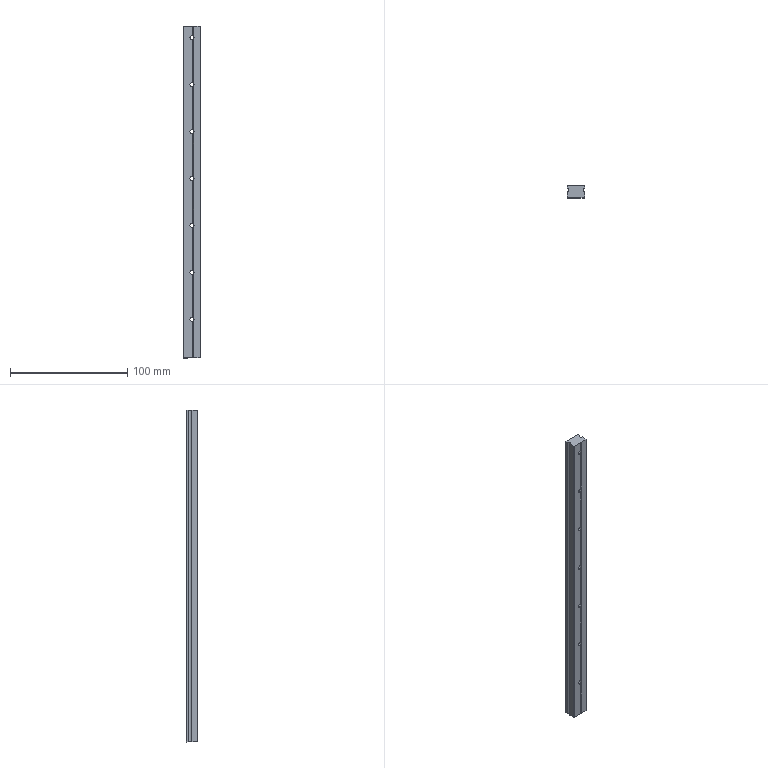Part | SolidWorks | features BaseBody 1 | 1 solid | 59 faces | box 15 x 10 x 283 mm | volume 39191 mm3 | cylinder 39 | plane 20 | commonest cylinder face diameters 3.5 x14 6 x14 0.6 x8 3 x3